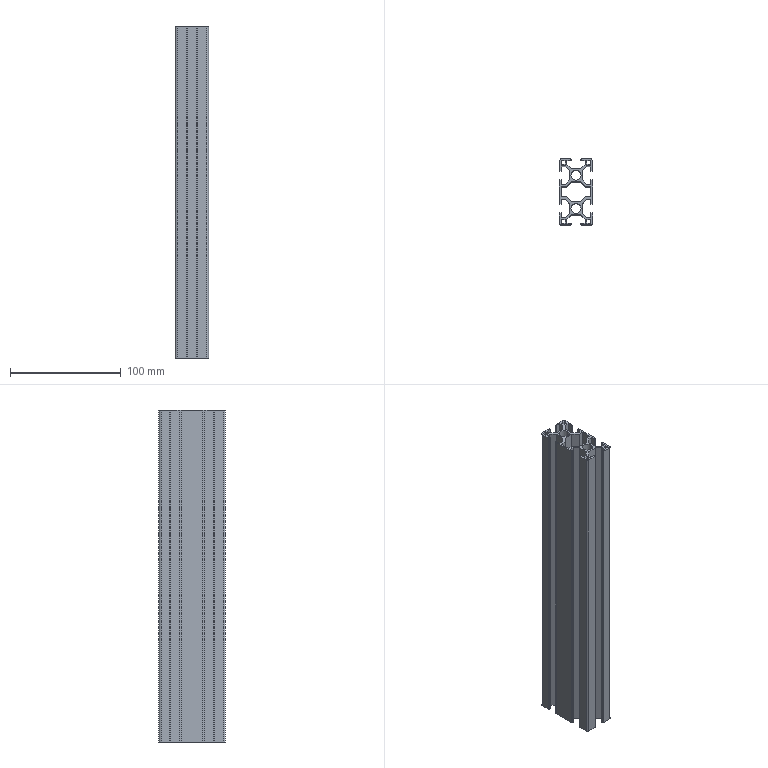Part | SolidWorks | features WeldMemberFeat 1, WeldmentFeature 1 | 1 solid | 126 faces | box 30 x 60 x 300 mm | volume 150091 mm3 | plane 118 | cylinder 8 | commonest cylinder face diameters 9.2 x4 3 x2 5 x2